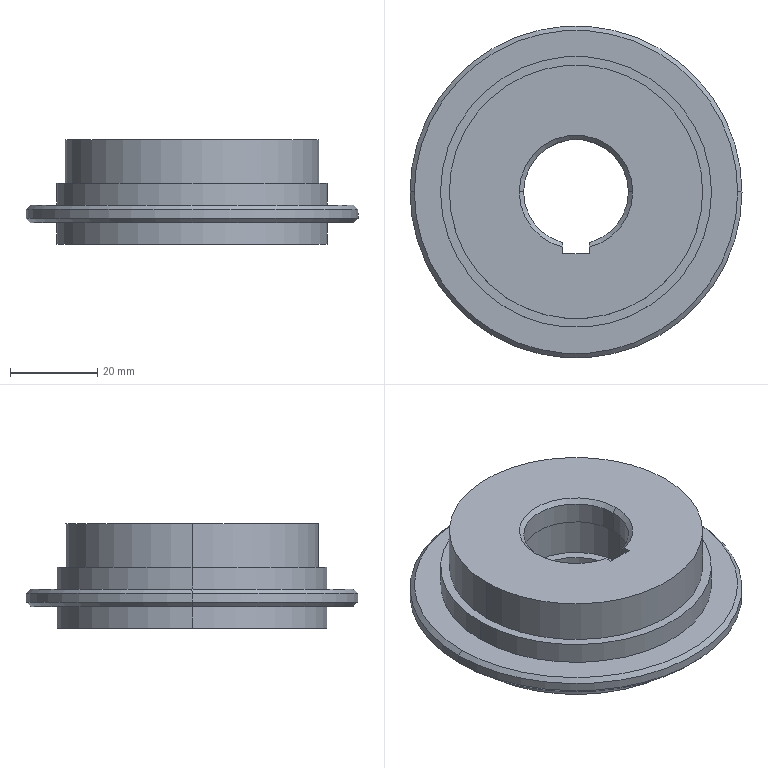Part | SolidWorks | features MirrorStock 1 | 2 solids | 49 faces | box 76 x 76 x 24 mm | volume 54312 mm3 | cylinder 25 | plane 14 | cone 10 | commonest cylinder face diameters 24 x6 58 x6 62 x4 28 x3 49 x2 52 x2
STEP:
#1=CARTESIAN_POINT('',(-12.,0.,21.));
#2=VERTEX_POINT('',#1);
#3=CARTESIAN_POINT('',(12.,0.,21.));
#4=VERTEX_POINT('',#3);
#5=CARTESIAN_POINT('',(0.,0.,21.));
#6=DIRECTION('',(0.,0.,-1.));
#7=DIRECTION('',(1.,0.,0.));
#8=AXIS2_PLACEMENT_3D('',#5,#6,#7);
#9=CIRCLE('',#8,12.);
#10=EDGE_CURVE('',#2,#4,#9,.T.);
#11=ORIENTED_EDGE('',*,*,#10,.T.);
#12=CARTESIAN_POINT('',(13.,0.,22.));
#13=VERTEX_POINT('',#12);
#14=CARTESIAN_POINT('',(13.,0.,22.));
#15=DIRECTION('',(0.7071,0.,0.7071));
#16=VECTOR('',#15,1000.);
#17=LINE('',#14,#16);
#18=EDGE_CURVE('',#4,#13,#17,.T.);
#19=ORIENTED_EDGE('',*,*,#18,.T.);
#20=CARTESIAN_POINT('',(-13.,0.,22.));
#21=VERTEX_POINT('',#20);
#22=CARTESIAN_POINT('',(0.,0.,22.));
#23=DIRECTION('',(0.,0.,1.));
#24=DIRECTION('',(1.,0.,0.));
#25=AXIS2_PLACEMENT_3D('',#22,#23,#24);
#26=CIRCLE('',#25,13.);
#27=EDGE_CURVE('',#13,#21,#26,.T.);
#28=ORIENTED_EDGE('',*,*,#27,.T.);
#29=CARTESIAN_POINT('',(-13.,0.,22.));
#30=DIRECTION('',(-0.7071,0.,0.7071));
#31=VECTOR('',#30,1000.);
#32=LINE('',#29,#31);
#33=EDGE_CURVE('',#2,#21,#32,.T.);
#34=ORIENTED_EDGE('',*,*,#33,.F.);
#35=EDGE_LOOP('',(#11,#19,#28,#34));
#36=FACE_OUTER_BOUND('',#35,.T.);
#37=CARTESIAN_POINT('',(0.,0.,22.));
#38=DIRECTION('',(0.,0.,1.));
#39=DIRECTION('',(-1.,0.,0.));
#40=AXIS2_PLACEMENT_3D('',#37,#38,#39);
#41=CONICAL_SURFACE('',#40,13.,0.7854);
#42=ADVANCED_FACE('',(#36),#41,.F.);
#43=CARTESIAN_POINT('',(-3.,-11.619,21.));
#44=VERTEX_POINT('',#43);
#45=CARTESIAN_POINT('',(0.,0.,21.));
#46=DIRECTION('',(0.,0.,-1.));
#47=DIRECTION('',(1.,0.,0.));
#48=AXIS2_PLACEMENT_3D('',#45,#46,#47);
#49=CIRCLE('',#48,12.);
#50=EDGE_CURVE('',#44,#2,#49,.T.);
#51=ORIENTED_EDGE('',*,*,#50,.T.);
#52=ORIENTED_EDGE('',*,*,#33,.T.);
#53=CARTESIAN_POINT('',(-3.,-12.649,22.));
#54=VERTEX_POINT('',#53);
#55=CARTESIAN_POINT('',(0.,0.,22.));
#56=DIRECTION('',(0.,0.,1.));
#57=DIRECTION('',(1.,0.,0.));
#58=AXIS2_PLACEMENT_3D('',#55,#56,#57);
#59=CIRCLE('',#58,13.);
#60=EDGE_CURVE('',#21,#54,#59,.T.);
#61=ORIENTED_EDGE('',*,*,#60,.T.);
#62=CARTESIAN_POINT('',(-3.,-12.649,22.));
#63=CARTESIAN_POINT('',(-3.,-12.306,21.666));
#64=CARTESIAN_POINT('',(-3.,-11.963,21.333));
#65=CARTESIAN_POINT('',(-3.,-11.619,21.));
#66=B_SPLINE_CURVE_WITH_KNOTS('',3,(#62,#63,#64,#65),.UNSPECIFIED.,.F.,.F.,(4,4),(0.,0.001436),.UNSPECIFIED.);
#67=EDGE_CURVE('',#54,#44,#66,.T.);
#68=ORIENTED_EDGE('',*,*,#67,.T.);
#69=EDGE_LOOP('',(#51,#52,#61,#68));
#70=FACE_OUTER_BOUND('',#69,.T.);
#71=CARTESIAN_POINT('',(0.,0.,22.));
#72=DIRECTION('',(0.,0.,1.));
#73=DIRECTION('',(-1.,0.,0.));
#74=AXIS2_PLACEMENT_3D('',#71,#72,#73);
#75=CONICAL_SURFACE('',#74,13.,0.7854);
#76=ADVANCED_FACE('',(#70),#75,.F.);
#77=CARTESIAN_POINT('',(12.,0.,1.));
#78=VERTEX_POINT('',#77);
#79=CARTESIAN_POINT('',(-12.,0.,1.));
#80=VERTEX_POINT('',#79);
#81=CARTESIAN_POINT('',(0.,0.,1.));
#82=DIRECTION('',(0.,0.,1.));
#83=DIRECTION('',(-1.,0.,0.));
#84=AXIS2_PLACEMENT_3D('',#81,#82,#83);
#85=CIRCLE('',#84,12.);
#86=EDGE_CURVE('',#78,#80,#85,.T.);
#87=ORIENTED_EDGE('',*,*,#86,.T.);
#88=CARTESIAN_POINT('',(-13.,0.,0.));
#89=VERTEX_POINT('',#88);
#90=CARTESIAN_POINT('',(-12.,0.,1.));
#91=DIRECTION('',(-0.7071,0.,-0.7071));
#92=VECTOR('',#91,1000.);
#93=LINE('',#90,#92);
#94=EDGE_CURVE('',#80,#89,#93,.T.);
#95=ORIENTED_EDGE('',*,*,#94,.T.);
#96=CARTESIAN_POINT('',(13.,0.,0.));
#97=VERTEX_POINT('',#96);
#98=CARTESIAN_POINT('',(0.,0.,0.));
#99=DIRECTION('',(0.,0.,-1.));
#100=DIRECTION('',(-1.,0.,0.));
#101=AXIS2_PLACEMENT_3D('',#98,#99,#100);
#102=CIRCLE('',#101,13.);
#103=EDGE_CURVE('',#89,#97,#102,.T.);
#104=ORIENTED_EDGE('',*,*,#103,.T.);
#105=CARTESIAN_POINT('',(12.,0.,1.));
#106=DIRECTION('',(0.7071,0.,-0.7071));
#107=VECTOR('',#106,1000.);
#108=LINE('',#105,#107);
#109=EDGE_CURVE('',#78,#97,#108,.T.);
#110=ORIENTED_EDGE('',*,*,#109,.F.);
#111=EDGE_LOOP('',(#87,#95,#104,#110));
#112=FACE_OUTER_BOUND('',#111,.T.);
#113=CARTESIAN_POINT('',(0.,0.,1.));
#114=DIRECTION('',(0.,0.,-1.));
#115=DIRECTION('',(1.,0.,0.));
#116=AXIS2_PLACEMENT_3D('',#113,#114,#115);
#117=CONICAL_SURFACE('',#116,12.,0.7854);
#118=ADVANCED_FACE('',(#112),#117,.F.);
#119=CARTESIAN_POINT('',(3.,-11.619,1.));
#120=VERTEX_POINT('',#119);
#121=CARTESIAN_POINT('',(0.,0.,1.));
#122=DIRECTION('',(0.,0.,1.));
#123=DIRECTION('',(-1.,0.,0.));
#124=AXIS2_PLACEMENT_3D('',#121,#122,#123);
#125=CIRCLE('',#124,12.);
#126=EDGE_CURVE('',#120,#78,#125,.T.);
#127=ORIENTED_EDGE('',*,*,#126,.T.);
#128=ORIENTED_EDGE('',*,*,#109,.T.);
#129=CARTESIAN_POINT('',(3.,-12.649,0.));
#130=VERTEX_POINT('',#129);
#131=CARTESIAN_POINT('',(0.,0.,0.));
#132=DIRECTION('',(0.,0.,-1.));
#133=DIRECTION('',(-1.,0.,0.));
#134=AXIS2_PLACEMENT_3D('',#131,#132,#133);
#135=CIRCLE('',#134,13.);
#136=EDGE_CURVE('',#97,#130,#135,.T.);
#137=ORIENTED_EDGE('',*,*,#136,.T.);
#138=CARTESIAN_POINT('',(3.,-12.649,0.));
#139=CARTESIAN_POINT('',(3.,-12.306,0.3337));
#140=CARTESIAN_POINT('',(3.,-11.963,0.6671));
#141=CARTESIAN_POINT('',(3.,-11.619,1.));
#142=B_SPLINE_CURVE_WITH_KNOTS('',3,(#138,#139,#140,#141),.UNSPECIFIED.,.F.,.F.,(4,4),(0.,0.001436),.UNSPECIFIED.);
#143=EDGE_CURVE('',#130,#120,#142,.T.);
#144=ORIENTED_EDGE('',*,*,#143,.T.);
#145=EDGE_LOOP('',(#127,#128,#137,#144));
#146=FACE_OUTER_BOUND('',#145,.T.);
#147=CARTESIAN_POINT('',(0.,0.,1.));
#148=DIRECTION('',(0.,0.,-1.));
#149=DIRECTION('',(1.,0.,0.));
#150=AXIS2_PLACEMENT_3D('',#147,#148,#149);
#151=CONICAL_SURFACE('',#150,12.,0.7854);
#152=ADVANCED_FACE('',(#146),#151,.F.);
#153=CARTESIAN_POINT('',(-29.,0.,22.));
#154=VERTEX_POINT('',#153);
#155=CARTESIAN_POINT('',(29.,0.,22.));
#156=VERTEX_POINT('',#155);
#157=CARTESIAN_POINT('',(0.,0.,22.));
#158=DIRECTION('',(0.,0.,1.));
#159=DIRECTION('',(1.,0.,0.));
#160=AXIS2_PLACEMENT_3D('',#157,#158,#159);
#161=CIRCLE('',#160,29.);
#162=EDGE_CURVE('',#154,#156,#161,.T.);
#163=ORIENTED_EDGE('',*,*,#162,.F.);
#164=CARTESIAN_POINT('',(-29.,0.,7.5));
#165=VERTEX_POINT('',#164);
#166=CARTESIAN_POINT('',(-29.,0.,0.));
#167=DIRECTION('',(0.,0.,-1.));
#168=VECTOR('',#167,1000.);
#169=LINE('',#166,#168);
#170=EDGE_CURVE('',#154,#165,#169,.T.);
#171=ORIENTED_EDGE('',*,*,#170,.T.);
#172=CARTESIAN_POINT('',(29.,0.,7.5));
#173=VERTEX_POINT('',#172);
#174=CARTESIAN_POINT('',(0.,0.,7.5));
#175=DIRECTION('',(0.,0.,1.));
#176=DIRECTION('',(1.,0.,0.));
#177=AXIS2_PLACEMENT_3D('',#174,#175,#176);
#178=CIRCLE('',#177,29.);
#179=EDGE_CURVE('',#165,#173,#178,.T.);
#180=ORIENTED_EDGE('',*,*,#179,.T.);
#181=CARTESIAN_POINT('',(29.,0.,0.));
#182=DIRECTION('',(0.,0.,-1.));
#183=VECTOR('',#182,1000.);
#184=LINE('',#181,#183);
#185=EDGE_CURVE('',#156,#173,#184,.T.);
#186=ORIENTED_EDGE('',*,*,#185,.F.);
#187=EDGE_LOOP('',(#163,#171,#180,#186));
#188=FACE_OUTER_BOUND('',#187,.T.);
#189=CARTESIAN_POINT('',(0.,0.,0.));
#190=DIRECTION('',(0.,0.,-1.));
#191=DIRECTION('',(1.,0.,0.));
#192=AXIS2_PLACEMENT_3D('',#189,#190,#191);
#193=CYLINDRICAL_SURFACE('',#192,29.);
#194=ADVANCED_FACE('',(#188),#193,.T.);
#195=CARTESIAN_POINT('',(-24.5,0.,7.5));
#196=VERTEX_POINT('',#195);
#197=CARTESIAN_POINT('',(24.5,0.,7.5));
#198=VERTEX_POINT('',#197);
#199=CARTESIAN_POINT('',(0.,0.,7.5));
#200=DIRECTION('',(0.,0.,1.));
#201=DIRECTION('',(1.,0.,0.));
#202=AXIS2_PLACEMENT_3D('',#199,#200,#201);
#203=CIRCLE('',#202,24.5);
#204=EDGE_CURVE('',#196,#198,#203,.T.);
#205=ORIENTED_EDGE('',*,*,#204,.F.);
#206=CARTESIAN_POINT('',(-24.5,0.,0.));
#207=VERTEX_POINT('',#206);
#208=CARTESIAN_POINT('',(-24.5,0.,0.));
#209=DIRECTION('',(0.,0.,-1.));
#210=VECTOR('',#209,1000.);
#211=LINE('',#208,#210);
#212=EDGE_CURVE('',#196,#207,#211,.T.);
#213=ORIENTED_EDGE('',*,*,#212,.T.);
#214=CARTESIAN_POINT('',(24.5,0.,0.));
#215=VERTEX_POINT('',#214);
#216=CARTESIAN_POINT('',(0.,0.,0.));
#217=DIRECTION('',(0.,0.,1.));
#218=DIRECTION('',(1.,0.,0.));
#219=AXIS2_PLACEMENT_3D('',#216,#217,#218);
#220=CIRCLE('',#219,24.5);
#221=EDGE_CURVE('',#207,#215,#220,.T.);
#222=ORIENTED_EDGE('',*,*,#221,.T.);
#223=CARTESIAN_POINT('',(24.5,0.,0.));
#224=DIRECTION('',(0.,0.,-1.));
#225=VECTOR('',#224,1000.);
#226=LINE('',#223,#225);
#227=EDGE_CURVE('',#198,#215,#226,.T.);
#228=ORIENTED_EDGE('',*,*,#227,.F.);
#229=EDGE_LOOP('',(#205,#213,#222,#228));
#230=FACE_OUTER_BOUND('',#229,.T.);
#231=CARTESIAN_POINT('',(0.,0.,0.));
#232=DIRECTION('',(0.,0.,-1.));
#233=DIRECTION('',(1.,0.,0.));
#234=AXIS2_PLACEMENT_3D('',#231,#232,#233);
#235=CYLINDRICAL_SURFACE('',#234,24.5);
#236=ADVANCED_FACE('',(#230),#235,.T.);
#237=CARTESIAN_POINT('',(12.,0.,6.));
#238=VERTEX_POINT('',#237);
#239=CARTESIAN_POINT('',(-12.,0.,6.));
#240=VERTEX_POINT('',#239);
#241=CARTESIAN_POINT('',(0.,0.,6.));
#242=DIRECTION('',(0.,0.,1.));
#243=DIRECTION('',(1.,0.,0.));
#244=AXIS2_PLACEMENT_3D('',#241,#242,#243);
#245=CIRCLE('',#244,12.);
#246=EDGE_CURVE('',#238,#240,#245,.T.);
#247=ORIENTED_EDGE('',*,*,#246,.T.);
#248=CARTESIAN_POINT('',(-12.,0.,0.));
#249=DIRECTION('',(0.,0.,-1.));
#250=VECTOR('',#249,1000.);
#251=LINE('',#248,#250);
#252=EDGE_CURVE('',#240,#80,#251,.T.);
#253=ORIENTED_EDGE('',*,*,#252,.T.);
#254=ORIENTED_EDGE('',*,*,#86,.F.);
#255=CARTESIAN_POINT('',(12.,0.,0.));
#256=DIRECTION('',(0.,0.,-1.));
#257=VECTOR('',#256,1000.);
#258=LINE('',#255,#257);
#259=EDGE_CURVE('',#238,#78,#258,.T.);
#260=ORIENTED_EDGE('',*,*,#259,.F.);
#261=EDGE_LOOP('',(#247,#253,#254,#260));
#262=FACE_OUTER_BOUND('',#261,.T.);
#263=CARTESIAN_POINT('',(0.,0.,0.));
#264=DIRECTION('',(0.,0.,-1.));
#265=DIRECTION('',(1.,0.,0.));
#266=AXIS2_PLACEMENT_3D('',#263,#264,#265);
#267=CYLINDRICAL_SURFACE('',#266,12.);
#268=ADVANCED_FACE('',(#262),#267,.F.);
#269=CARTESIAN_POINT('',(3.,-11.619,6.));
#270=VERTEX_POINT('',#269);
#271=CARTESIAN_POINT('',(0.,0.,6.));
#272=DIRECTION('',(0.,0.,1.));
#273=DIRECTION('',(1.,0.,0.));
#274=AXIS2_PLACEMENT_3D('',#271,#272,#273);
#275=CIRCLE('',#274,12.);
#276=EDGE_CURVE('',#270,#238,#275,.T.);
#277=ORIENTED_EDGE('',*,*,#276,.T.);
#278=ORIENTED_EDGE('',*,*,#259,.T.);
#279=ORIENTED_EDGE('',*,*,#126,.F.);
#280=CARTESIAN_POINT('',(3.,-11.619,0.));
#281=DIRECTION('',(0.,0.,-1.));
#282=VECTOR('',#281,1000.);
#283=LINE('',#280,#282);
#284=EDGE_CURVE('',#270,#120,#283,.T.);
#285=ORIENTED_EDGE('',*,*,#284,.F.);
#286=EDGE_LOOP('',(#277,#278,#279,#285));
#287=FACE_OUTER_BOUND('',#286,.T.);
#288=CARTESIAN_POINT('',(0.,0.,0.));
#289=DIRECTION('',(0.,0.,-1.));
#290=DIRECTION('',(1.,0.,0.));
#291=AXIS2_PLACEMENT_3D('',#288,#289,#290);
#292=CYLINDRICAL_SURFACE('',#291,12.);
#293=ADVANCED_FACE('',(#287),#292,.F.);
#294=CARTESIAN_POINT('',(14.,0.,16.));
#295=VERTEX_POINT('',#294);
#296=CARTESIAN_POINT('',(-14.,0.,16.));
#297=VERTEX_POINT('',#296);
#298=CARTESIAN_POINT('',(0.,0.,16.));
#299=DIRECTION('',(0.,0.,1.));
#300=DIRECTION('',(1.,0.,0.));
#301=AXIS2_PLACEMENT_3D('',#298,#299,#300);
#302=CIRCLE('',#301,14.);
#303=EDGE_CURVE('',#295,#297,#302,.T.);
#304=ORIENTED_EDGE('',*,*,#303,.T.);
#305=CARTESIAN_POINT('',(-14.,0.,6.));
#306=VERTEX_POINT('',#305);
#307=CARTESIAN_POINT('',(-14.,0.,0.));
#308=DIRECTION('',(0.,0.,-1.));
#309=VECTOR('',#308,1000.);
#310=LINE('',#307,#309);
#311=EDGE_CURVE('',#297,#306,#310,.T.);
#312=ORIENTED_EDGE('',*,*,#311,.T.);
#313=CARTESIAN_POINT('',(14.,0.,6.));
#314=VERTEX_POINT('',#313);
#315=CARTESIAN_POINT('',(0.,0.,6.));
#316=DIRECTION('',(0.,0.,1.));
#317=DIRECTION('',(1.,0.,0.));
#318=AXIS2_PLACEMENT_3D('',#315,#316,#317);
#319=CIRCLE('',#318,14.);
#320=EDGE_CURVE('',#314,#306,#319,.T.);
#321=ORIENTED_EDGE('',*,*,#320,.F.);
#322=CARTESIAN_POINT('',(14.,0.,0.));
#323=DIRECTION('',(0.,0.,-1.));
#324=VECTOR('',#323,1000.);
#325=LINE('',#322,#324);
#326=EDGE_CURVE('',#295,#314,#325,.T.);
#327=ORIENTED_EDGE('',*,*,#326,.F.);
#328=EDGE_LOOP('',(#304,#312,#321,#327));
#329=FACE_OUTER_BOUND('',#328,.T.);
#330=CARTESIAN_POINT('',(0.,0.,0.));
#331=DIRECTION('',(0.,0.,-1.));
#332=DIRECTION('',(1.,0.,0.));
#333=AXIS2_PLACEMENT_3D('',#330,#331,#332);
#334=CYLINDRICAL_SURFACE('',#333,14.);
#335=ADVANCED_FACE('',(#329),#334,.F.);
#336=CARTESIAN_POINT('',(3.,-13.675,16.));
#337=VERTEX_POINT('',#336);
#338=CARTESIAN_POINT('',(0.,0.,16.));
#339=DIRECTION('',(0.,0.,1.));
#340=DIRECTION('',(1.,0.,0.));
#341=AXIS2_PLACEMENT_3D('',#338,#339,#340);
#342=CIRCLE('',#341,14.);
#343=EDGE_CURVE('',#337,#295,#342,.T.);
#344=ORIENTED_EDGE('',*,*,#343,.T.);
#345=ORIENTED_EDGE('',*,*,#326,.T.);
#346=CARTESIAN_POINT('',(3.,-13.675,6.));
#347=VERTEX_POINT('',#346);
#348=CARTESIAN_POINT('',(0.,0.,6.));
#349=DIRECTION('',(0.,0.,1.));
#350=DIRECTION('',(1.,0.,0.));
#351=AXIS2_PLACEMENT_3D('',#348,#349,#350);
#352=CIRCLE('',#351,14.);
#353=EDGE_CURVE('',#347,#314,#352,.T.);
#354=ORIENTED_EDGE('',*,*,#353,.F.);
#355=CARTESIAN_POINT('',(3.,-13.675,0.));
#356=DIRECTION('',(0.,0.,-1.));
#357=VECTOR('',#356,1000.);
#358=LINE('',#355,#357);
#359=EDGE_CURVE('',#337,#347,#358,.T.);
#360=ORIENTED_EDGE('',*,*,#359,.F.);
#361=EDGE_LOOP('',(#344,#345,#354,#360));
#362=FACE_OUTER_BOUND('',#361,.T.);
#363=CARTESIAN_POINT('',(0.,0.,0.));
#364=DIRECTION('',(0.,0.,-1.));
#365=DIRECTION('',(1.,0.,0.));
#366=AXIS2_PLACEMENT_3D('',#363,#364,#365);
#367=CYLINDRICAL_SURFACE('',#366,14.);
#368=ADVANCED_FACE('',(#362),#367,.F.);
#369=ORIENTED_EDGE('',*,*,#10,.F.);
#370=CARTESIAN_POINT('',(-12.,0.,16.));
#371=VERTEX_POINT('',#370);
#372=CARTESIAN_POINT('',(-12.,0.,0.));
#373=DIRECTION('',(0.,0.,-1.));
#374=VECTOR('',#373,1000.);
#375=LINE('',#372,#374);
#376=EDGE_CURVE('',#2,#371,#375,.T.);
#377=ORIENTED_EDGE('',*,*,#376,.T.);
#378=CARTESIAN_POINT('',(12.,0.,16.));
#379=VERTEX_POINT('',#378);
#380=CARTESIAN_POINT('',(0.,0.,16.));
#381=DIRECTION('',(0.,0.,1.));
#382=DIRECTION('',(1.,0.,0.));
#383=AXIS2_PLACEMENT_3D('',#380,#381,#382);
#384=CIRCLE('',#383,12.);
#385=EDGE_CURVE('',#379,#371,#384,.T.);
#386=ORIENTED_EDGE('',*,*,#385,.F.);
#387=CARTESIAN_POINT('',(12.,0.,0.));
#388=DIRECTION('',(0.,0.,-1.));
#389=VECTOR('',#388,1000.);
#390=LINE('',#387,#389);
#391=EDGE_CURVE('',#4,#379,#390,.T.);
#392=ORIENTED_EDGE('',*,*,#391,.F.);
#393=EDGE_LOOP('',(#369,#377,#386,#392));
#394=FACE_OUTER_BOUND('',#393,.T.);
#395=CARTESIAN_POINT('',(0.,0.,0.));
#396=DIRECTION('',(0.,0.,-1.));
#397=DIRECTION('',(1.,0.,0.));
#398=AXIS2_PLACEMENT_3D('',#395,#396,#397);
#399=CYLINDRICAL_SURFACE('',#398,12.);
#400=ADVANCED_FACE('',(#394),#399,.F.);
#401=CARTESIAN_POINT('',(3.,-11.619,21.));
#402=VERTEX_POINT('',#401);
#403=CARTESIAN_POINT('',(0.,0.,21.));
#404=DIRECTION('',(0.,0.,-1.));
#405=DIRECTION('',(1.,0.,0.));
#406=AXIS2_PLACEMENT_3D('',#403,#404,#405);
#407=CIRCLE('',#406,12.);
#408=EDGE_CURVE('',#4,#402,#407,.T.);
#409=ORIENTED_EDGE('',*,*,#408,.F.);
#410=ORIENTED_EDGE('',*,*,#391,.T.);
#411=CARTESIAN_POINT('',(3.,-11.619,16.));
#412=VERTEX_POINT('',#411);
#413=CARTESIAN_POINT('',(0.,0.,16.));
#414=DIRECTION('',(0.,0.,1.));
#415=DIRECTION('',(1.,0.,0.));
#416=AXIS2_PLACEMENT_3D('',#413,#414,#415);
#417=CIRCLE('',#416,12.);
#418=EDGE_CURVE('',#412,#379,#417,.T.);
#419=ORIENTED_EDGE('',*,*,#418,.F.);
#420=CARTESIAN_POINT('',(3.,-11.619,0.));
#421=DIRECTION('',(0.,0.,-1.));
#422=VECTOR('',#421,1000.);
#423=LINE('',#420,#422);
#424=EDGE_CURVE('',#402,#412,#423,.T.);
#425=ORIENTED_EDGE('',*,*,#424,.F.);
#426=EDGE_LOOP('',(#409,#410,#419,#425));
#427=FACE_OUTER_BOUND('',#426,.T.);
#428=CARTESIAN_POINT('',(0.,0.,0.));
#429=DIRECTION('',(0.,0.,-1.));
#430=DIRECTION('',(1.,0.,0.));
#431=AXIS2_PLACEMENT_3D('',#428,#429,#430);
#432=CYLINDRICAL_SURFACE('',#431,12.);
#433=ADVANCED_FACE('',(#427),#432,.F.);
#434=CARTESIAN_POINT('',(0.,0.,22.));
#435=DIRECTION('',(0.,0.,1.));
#436=DIRECTION('',(1.,0.,0.));
#437=AXIS2_PLACEMENT_3D('',#434,#435,#436);
#438=CIRCLE('',#437,29.);
#439=EDGE_CURVE('',#156,#154,#438,.T.);
#440=ORIENTED_EDGE('',*,*,#439,.T.);
#441=ORIENTED_EDGE('',*,*,#162,.T.);
#442=EDGE_LOOP('',(#440,#441));
#443=FACE_OUTER_BOUND('',#442,.T.);
#444=CARTESIAN_POINT('',(3.,-12.649,22.));
#445=VERTEX_POINT('',#444);
#446=CARTESIAN_POINT('',(3.,-14.2,22.));
#447=VERTEX_POINT('',#446);
#448=CARTESIAN_POINT('',(3.,-14.2,22.));
#449=DIRECTION('',(0.,-1.,0.));
#450=VECTOR('',#449,1000.);
#451=LINE('',#448,#450);
#452=EDGE_CURVE('',#445,#447,#451,.T.);
#453=ORIENTED_EDGE('',*,*,#452,.T.);
#454=CARTESIAN_POINT('',(-3.,-14.2,22.));
#455=VERTEX_POINT('',#454);
#456=CARTESIAN_POINT('',(-3.,-14.2,22.));
#457=DIRECTION('',(-1.,0.,0.));
#458=VECTOR('',#457,1000.);
#459=LINE('',#456,#458);
#460=EDGE_CURVE('',#447,#455,#459,.T.);
#461=ORIENTED_EDGE('',*,*,#460,.T.);
#462=CARTESIAN_POINT('',(-3.,-14.2,22.));
#463=DIRECTION('',(0.,1.,0.));
#464=VECTOR('',#463,1000.);
#465=LINE('',#462,#464);
#466=EDGE_CURVE('',#455,#54,#465,.T.);
#467=ORIENTED_EDGE('',*,*,#466,.T.);
#468=ORIENTED_EDGE('',*,*,#60,.F.);
#469=ORIENTED_EDGE('',*,*,#27,.F.);
#470=CARTESIAN_POINT('',(0.,0.,22.));
#471=DIRECTION('',(0.,0.,1.));
#472=DIRECTION('',(1.,0.,0.));
#473=AXIS2_PLACEMENT_3D('',#470,#471,#472);
#474=CIRCLE('',#473,13.);
#475=EDGE_CURVE('',#445,#13,#474,.T.);
#476=ORIENTED_EDGE('',*,*,#475,.F.);
#477=EDGE_LOOP('',(#453,#461,#467,#468,#469,#476));
#478=FACE_BOUND('',#477,.T.);
#479=CARTESIAN_POINT('',(-29.,0.,22.));
#480=DIRECTION('',(0.,0.,-1.));
#481=DIRECTION('',(1.,0.,0.));
#482=AXIS2_PLACEMENT_3D('',#479,#480,#481);
#483=PLANE('',#482);
#484=ADVANCED_FACE('',(#443,#478),#483,.F.);
#485=ORIENTED_EDGE('',*,*,#376,.F.);
#486=ORIENTED_EDGE('',*,*,#50,.F.);
#487=CARTESIAN_POINT('',(-3.,-11.619,16.));
#488=VERTEX_POINT('',#487);
#489=CARTESIAN_POINT('',(-3.,-11.619,0.));
#490=DIRECTION('',(0.,0.,1.));
#491=VECTOR('',#490,1000.);
#492=LINE('',#489,#491);
#493=EDGE_CURVE('',#488,#44,#492,.T.);
#494=ORIENTED_EDGE('',*,*,#493,.F.);
#495=CARTESIAN_POINT('',(0.,0.,16.));
#496=DIRECTION('',(0.,0.,1.));
#497=DIRECTION('',(1.,0.,0.));
#498=AXIS2_PLACEMENT_3D('',#495,#496,#497);
#499=CIRCLE('',#498,12.);
#500=EDGE_CURVE('',#371,#488,#499,.T.);
#501=ORIENTED_EDGE('',*,*,#500,.F.);
#502=EDGE_LOOP('',(#485,#486,#494,#501));
#503=FACE_OUTER_BOUND('',#502,.T.);
#504=CARTESIAN_POINT('',(0.,0.,0.));
#505=DIRECTION('',(0.,0.,-1.));
#506=DIRECTION('',(1.,0.,0.));
#507=AXIS2_PLACEMENT_3D('',#504,#505,#506);
#508=CYLINDRICAL_SURFACE('',#507,12.);
#509=ADVANCED_FACE('',(#503),#508,.F.);
#510=ORIENTED_EDGE('',*,*,#418,.T.);
#511=ORIENTED_EDGE('',*,*,#385,.T.);
#512=ORIENTED_EDGE('',*,*,#500,.T.);
#513=CARTESIAN_POINT('',(-3.,-13.675,16.));
#514=VERTEX_POINT('',#513);
#515=CARTESIAN_POINT('',(-3.,0.,16.));
#516=DIRECTION('',(0.,1.,0.));
#517=VECTOR('',#516,1000.);
#518=LINE('',#515,#517);
#519=EDGE_CURVE('',#514,#488,#518,.T.);
#520=ORIENTED_EDGE('',*,*,#519,.F.);
#521=CARTESIAN_POINT('',(0.,0.,16.));
#522=DIRECTION('',(0.,0.,1.));
#523=DIRECTION('',(1.,0.,0.));
#524=AXIS2_PLACEMENT_3D('',#521,#522,#523);
#525=CIRCLE('',#524,14.);
#526=EDGE_CURVE('',#297,#514,#525,.T.);
#527=ORIENTED_EDGE('',*,*,#526,.F.);
#528=ORIENTED_EDGE('',*,*,#303,.F.);
#529=ORIENTED_EDGE('',*,*,#343,.F.);
#530=CARTESIAN_POINT('',(3.,0.,16.));
#531=DIRECTION('',(0.,-1.,0.));
#532=VECTOR('',#531,1000.);
#533=LINE('',#530,#532);
#534=EDGE_CURVE('',#412,#337,#533,.T.);
#535=ORIENTED_EDGE('',*,*,#534,.F.);
#536=EDGE_LOOP('',(#510,#511,#512,#520,#527,#528,#529,#535));
#537=FACE_OUTER_BOUND('',#536,.T.);
#538=CARTESIAN_POINT('',(-12.,0.,16.));
#539=DIRECTION('',(0.,0.,1.));
#540=DIRECTION('',(-1.,0.,0.));
#541=AXIS2_PLACEMENT_3D('',#538,#539,#540);
#542=PLANE('',#541);
#543=ADVANCED_FACE('',(#537),#542,.F.);
#544=ORIENTED_EDGE('',*,*,#311,.F.);
#545=ORIENTED_EDGE('',*,*,#526,.T.);
#546=CARTESIAN_POINT('',(-3.,-13.675,6.));
#547=VERTEX_POINT('',#546);
#548=CARTESIAN_POINT('',(-3.,-13.675,0.));
#549=DIRECTION('',(0.,0.,1.));
#550=VECTOR('',#549,1000.);
#551=LINE('',#548,#550);
#552=EDGE_CURVE('',#547,#514,#551,.T.);
#553=ORIENTED_EDGE('',*,*,#552,.F.);
#554=CARTESIAN_POINT('',(0.,0.,6.));
#555=DIRECTION('',(0.,0.,1.));
#556=DIRECTION('',(1.,0.,0.));
#557=AXIS2_PLACEMENT_3D('',#554,#555,#556);
#558=CIRCLE('',#557,14.);
#559=EDGE_CURVE('',#306,#547,#558,.T.);
#560=ORIENTED_EDGE('',*,*,#559,.F.);
#561=EDGE_LOOP('',(#544,#545,#553,#560));
#562=FACE_OUTER_BOUND('',#561,.T.);
#563=CARTESIAN_POINT('',(0.,0.,0.));
#564=DIRECTION('',(0.,0.,-1.));
#565=DIRECTION('',(1.,0.,0.));
#566=AXIS2_PLACEMENT_3D('',#563,#564,#565);
#567=CYLINDRICAL_SURFACE('',#566,14.);
#568=ADVANCED_FACE('',(#562),#567,.F.);
#569=ORIENTED_EDGE('',*,*,#353,.T.);
#570=ORIENTED_EDGE('',*,*,#320,.T.);
#571=ORIENTED_EDGE('',*,*,#559,.T.);
#572=CARTESIAN_POINT('',(-3.,-11.619,6.));
#573=VERTEX_POINT('',#572);
#574=CARTESIAN_POINT('',(-3.,0.,6.));
#575=DIRECTION('',(0.,-1.,0.));
#576=VECTOR('',#575,1000.);
#577=LINE('',#574,#576);
#578=EDGE_CURVE('',#573,#547,#577,.T.);
#579=ORIENTED_EDGE('',*,*,#578,.F.);
#580=CARTESIAN_POINT('',(0.,0.,6.));
#581=DIRECTION('',(0.,0.,1.));
#582=DIRECTION('',(1.,0.,0.));
#583=AXIS2_PLACEMENT_3D('',#580,#581,#582);
#584=CIRCLE('',#583,12.);
#585=EDGE_CURVE('',#240,#573,#584,.T.);
#586=ORIENTED_EDGE('',*,*,#585,.F.);
#587=ORIENTED_EDGE('',*,*,#246,.F.);
#588=ORIENTED_EDGE('',*,*,#276,.F.);
#589=CARTESIAN_POINT('',(3.,0.,6.));
#590=DIRECTION('',(0.,1.,0.));
#591=VECTOR('',#590,1000.);
#592=LINE('',#589,#591);
#593=EDGE_CURVE('',#347,#270,#592,.T.);
#594=ORIENTED_EDGE('',*,*,#593,.F.);
#595=EDGE_LOOP('',(#569,#570,#571,#579,#586,#587,#588,#594));
#596=FACE_OUTER_BOUND('',#595,.T.);
#597=CARTESIAN_POINT('',(-14.,0.,6.));
#598=DIRECTION('',(0.,0.,-1.));
#599=DIRECTION('',(1.,0.,0.));
#600=AXIS2_PLACEMENT_3D('',#597,#598,#599);
#601=PLANE('',#600);
#602=ADVANCED_FACE('',(#596),#601,.F.);
#603=ORIENTED_EDGE('',*,*,#252,.F.);
#604=ORIENTED_EDGE('',*,*,#585,.T.);
#605=CARTESIAN_POINT('',(-3.,-11.619,1.));
#606=VERTEX_POINT('',#605);
#607=CARTESIAN_POINT('',(-3.,-11.619,0.));
#608=DIRECTION('',(0.,0.,1.));
#609=VECTOR('',#608,1000.);
#610=LINE('',#607,#609);
#611=EDGE_CURVE('',#606,#573,#610,.T.);
#612=ORIENTED_EDGE('',*,*,#611,.F.);
#613=CARTESIAN_POINT('',(0.,0.,1.));
#614=DIRECTION('',(0.,0.,1.));
#615=DIRECTION('',(-1.,0.,0.));
#616=AXIS2_PLACEMENT_3D('',#613,#614,#615);
#617=CIRCLE('',#616,12.);
#618=EDGE_CURVE('',#80,#606,#617,.T.);
#619=ORIENTED_EDGE('',*,*,#618,.F.);
#620=EDGE_LOOP('',(#603,#604,#612,#619));
#621=FACE_OUTER_BOUND('',#620,.T.);
#622=CARTESIAN_POINT('',(0.,0.,0.));
#623=DIRECTION('',(0.,0.,-1.));
#624=DIRECTION('',(1.,0.,0.));
#625=AXIS2_PLACEMENT_3D('',#622,#623,#624);
#626=CYLINDRICAL_SURFACE('',#625,12.);
#627=ADVANCED_FACE('',(#621),#626,.F.);
#628=CARTESIAN_POINT('',(-3.,-14.2,0.));
#629=VERTEX_POINT('',#628);
#630=CARTESIAN_POINT('',(-3.,-12.649,0.));
#631=VERTEX_POINT('',#630);
#632=CARTESIAN_POINT('',(-3.,0.,0.));
#633=DIRECTION('',(0.,1.,0.));
#634=VECTOR('',#633,1000.);
#635=LINE('',#632,#634);
#636=EDGE_CURVE('',#629,#631,#635,.T.);
#637=ORIENTED_EDGE('',*,*,#636,.F.);
#638=CARTESIAN_POINT('',(3.,-14.2,0.));
#639=VERTEX_POINT('',#638);
#640=CARTESIAN_POINT('',(-12.,-14.2,0.));
#641=DIRECTION('',(-1.,0.,0.));
#642=VECTOR('',#641,1000.);
#643=LINE('',#640,#642);
#644=EDGE_CURVE('',#639,#629,#643,.T.);
#645=ORIENTED_EDGE('',*,*,#644,.F.);
#646=CARTESIAN_POINT('',(3.,0.,0.));
#647=DIRECTION('',(0.,-1.,0.));
#648=VECTOR('',#647,1000.);
#649=LINE('',#646,#648);
#650=EDGE_CURVE('',#130,#639,#649,.T.);
#651=ORIENTED_EDGE('',*,*,#650,.F.);
#652=ORIENTED_EDGE('',*,*,#136,.F.);
#653=ORIENTED_EDGE('',*,*,#103,.F.);
#654=CARTESIAN_POINT('',(0.,0.,0.));
#655=DIRECTION('',(0.,0.,-1.));
#656=DIRECTION('',(-1.,0.,0.));
#657=AXIS2_PLACEMENT_3D('',#654,#655,#656);
#658=CIRCLE('',#657,13.);
#659=EDGE_CURVE('',#631,#89,#658,.T.);
#660=ORIENTED_EDGE('',*,*,#659,.F.);
#661=EDGE_LOOP('',(#637,#645,#651,#652,#653,#660));
#662=FACE_BOUND('',#661,.T.);
#663=CARTESIAN_POINT('',(0.,0.,0.));
#664=DIRECTION('',(0.,0.,1.));
#665=DIRECTION('',(1.,0.,0.));
#666=AXIS2_PLACEMENT_3D('',#663,#664,#665);
#667=CIRCLE('',#666,24.5);
#668=EDGE_CURVE('',#215,#207,#667,.T.);
#669=ORIENTED_EDGE('',*,*,#668,.F.);
#670=ORIENTED_EDGE('',*,*,#221,.F.);
#671=EDGE_LOOP('',(#669,#670));
#672=FACE_OUTER_BOUND('',#671,.T.);
#673=CARTESIAN_POINT('',(-12.,0.,0.));
#674=DIRECTION('',(0.,0.,1.));
#675=DIRECTION('',(-1.,0.,0.));
#676=AXIS2_PLACEMENT_3D('',#673,#674,#675);
#677=PLANE('',#676);
#678=ADVANCED_FACE('',(#662,#672),#677,.F.);
#679=ORIENTED_EDGE('',*,*,#212,.F.);
#680=CARTESIAN_POINT('',(0.,0.,7.5));
#681=DIRECTION('',(0.,0.,1.));
#682=DIRECTION('',(1.,0.,0.));
#683=AXIS2_PLACEMENT_3D('',#680,#681,#682);
#684=CIRCLE('',#683,24.5);
#685=EDGE_CURVE('',#198,#196,#684,.T.);
#686=ORIENTED_EDGE('',*,*,#685,.F.);
#687=ORIENTED_EDGE('',*,*,#227,.T.);
#688=ORIENTED_EDGE('',*,*,#668,.T.);
#689=EDGE_LOOP('',(#679,#686,#687,#688));
#690=FACE_OUTER_BOUND('',#689,.T.);
#691=CARTESIAN_POINT('',(0.,0.,0.));
#692=DIRECTION('',(0.,0.,-1.));
#693=DIRECTION('',(1.,0.,0.));
#694=AXIS2_PLACEMENT_3D('',#691,#692,#693);
#695=CYLINDRICAL_SURFACE('',#694,24.5);
#696=ADVANCED_FACE('',(#690),#695,.T.);
#697=ORIENTED_EDGE('',*,*,#685,.T.);
#698=ORIENTED_EDGE('',*,*,#204,.T.);
#699=EDGE_LOOP('',(#697,#698));
#700=FACE_BOUND('',#699,.T.);
#701=CARTESIAN_POINT('',(0.,0.,7.5));
#702=DIRECTION('',(0.,0.,1.));
#703=DIRECTION('',(1.,0.,0.));
#704=AXIS2_PLACEMENT_3D('',#701,#702,#703);
#705=CIRCLE('',#704,29.);
#706=EDGE_CURVE('',#173,#165,#705,.T.);
#707=ORIENTED_EDGE('',*,*,#706,.F.);
#708=ORIENTED_EDGE('',*,*,#179,.F.);
#709=EDGE_LOOP('',(#707,#708));
#710=FACE_OUTER_BOUND('',#709,.T.);
#711=CARTESIAN_POINT('',(-24.5,0.,7.5));
#712=DIRECTION('',(0.,0.,1.));
#713=DIRECTION('',(-1.,0.,0.));
#714=AXIS2_PLACEMENT_3D('',#711,#712,#713);
#715=PLANE('',#714);
#716=ADVANCED_FACE('',(#700,#710),#715,.F.);
#717=ORIENTED_EDGE('',*,*,#170,.F.);
#718=ORIENTED_EDGE('',*,*,#439,.F.);
#719=ORIENTED_EDGE('',*,*,#185,.T.);
#720=ORIENTED_EDGE('',*,*,#706,.T.);
#721=EDGE_LOOP('',(#717,#718,#719,#720));
#722=FACE_OUTER_BOUND('',#721,.T.);
#723=CARTESIAN_POINT('',(0.,0.,0.));
#724=DIRECTION('',(0.,0.,-1.));
#725=DIRECTION('',(1.,0.,0.));
#726=AXIS2_PLACEMENT_3D('',#723,#724,#725);
#727=CYLINDRICAL_SURFACE('',#726,29.);
#728=ADVANCED_FACE('',(#722),#727,.T.);
#729=ORIENTED_EDGE('',*,*,#650,.T.);
#730=CARTESIAN_POINT('',(3.,-14.2,-2.));
#731=DIRECTION('',(0.,0.,1.));
#732=VECTOR('',#731,1000.);
#733=LINE('',#730,#732);
#734=EDGE_CURVE('',#639,#447,#733,.T.);
#735=ORIENTED_EDGE('',*,*,#734,.T.);
#736=ORIENTED_EDGE('',*,*,#452,.F.);
#737=CARTESIAN_POINT('',(3.,-11.619,21.));
#738=CARTESIAN_POINT('',(3.,-11.963,21.333));
#739=CARTESIAN_POINT('',(3.,-12.306,21.666));
#740=CARTESIAN_POINT('',(3.,-12.649,22.));
#741=B_SPLINE_CURVE_WITH_KNOTS('',3,(#737,#738,#739,#740),.UNSPECIFIED.,.F.,.F.,(4,4),(0.,0.001436),.UNSPECIFIED.);
#742=EDGE_CURVE('',#402,#445,#741,.T.);
#743=ORIENTED_EDGE('',*,*,#742,.F.);
#744=ORIENTED_EDGE('',*,*,#424,.T.);
#745=ORIENTED_EDGE('',*,*,#534,.T.);
#746=ORIENTED_EDGE('',*,*,#359,.T.);
#747=ORIENTED_EDGE('',*,*,#593,.T.);
#748=ORIENTED_EDGE('',*,*,#284,.T.);
#749=ORIENTED_EDGE('',*,*,#143,.F.);
#750=EDGE_LOOP('',(#729,#735,#736,#743,#744,#745,#746,#747,#748,#749));
#751=FACE_OUTER_BOUND('',#750,.T.);
#752=CARTESIAN_POINT('',(3.,-14.2,-2.));
#753=DIRECTION('',(1.,0.,0.));
#754=DIRECTION('',(0.,0.,1.));
#755=AXIS2_PLACEMENT_3D('',#752,#753,#754);
#756=PLANE('',#755);
#757=ADVANCED_FACE('',(#751),#756,.F.);
#758=ORIENTED_EDGE('',*,*,#611,.T.);
#759=ORIENTED_EDGE('',*,*,#578,.T.);
#760=ORIENTED_EDGE('',*,*,#552,.T.);
#761=ORIENTED_EDGE('',*,*,#519,.T.);
#762=ORIENTED_EDGE('',*,*,#493,.T.);
#763=ORIENTED_EDGE('',*,*,#67,.F.);
#764=ORIENTED_EDGE('',*,*,#466,.F.);
#765=CARTESIAN_POINT('',(-3.,-14.2,-2.));
#766=DIRECTION('',(0.,0.,1.));
#767=VECTOR('',#766,1000.);
#768=LINE('',#765,#767);
#769=EDGE_CURVE('',#629,#455,#768,.T.);
#770=ORIENTED_EDGE('',*,*,#769,.F.);
#771=ORIENTED_EDGE('',*,*,#636,.T.);
#772=CARTESIAN_POINT('',(-3.,-11.619,1.));
#773=CARTESIAN_POINT('',(-3.,-11.963,0.6671));
#774=CARTESIAN_POINT('',(-3.,-12.306,0.3337));
#775=CARTESIAN_POINT('',(-3.,-12.649,0.));
#776=B_SPLINE_CURVE_WITH_KNOTS('',3,(#772,#773,#774,#775),.UNSPECIFIED.,.F.,.F.,(4,4),(0.,0.001436),.UNSPECIFIED.);
#777=EDGE_CURVE('',#606,#631,#776,.T.);
#778=ORIENTED_EDGE('',*,*,#777,.F.);
#779=EDGE_LOOP('',(#758,#759,#760,#761,#762,#763,#764,#770,#771,#778));
#780=FACE_OUTER_BOUND('',#779,.T.);
#781=CARTESIAN_POINT('',(-3.,-14.2,-2.));
#782=DIRECTION('',(-1.,0.,0.));
#783=DIRECTION('',(0.,0.,-1.));
#784=AXIS2_PLACEMENT_3D('',#781,#782,#783);
#785=PLANE('',#784);
#786=ADVANCED_FACE('',(#780),#785,.F.);
#787=ORIENTED_EDGE('',*,*,#734,.F.);
#788=ORIENTED_EDGE('',*,*,#644,.T.);
#789=ORIENTED_EDGE('',*,*,#769,.T.);
#790=ORIENTED_EDGE('',*,*,#460,.F.);
#791=EDGE_LOOP('',(#787,#788,#789,#790));
#792=FACE_OUTER_BOUND('',#791,.T.);
#793=CARTESIAN_POINT('',(-3.,-14.2,-2.));
#794=DIRECTION('',(0.,-1.,0.));
#795=DIRECTION('',(0.,0.,1.));
#796=AXIS2_PLACEMENT_3D('',#793,#794,#795);
#797=PLANE('',#796);
#798=ADVANCED_FACE('',(#792),#797,.F.);
#799=ORIENTED_EDGE('',*,*,#94,.F.);
#800=ORIENTED_EDGE('',*,*,#618,.T.);
#801=ORIENTED_EDGE('',*,*,#777,.T.);
#802=ORIENTED_EDGE('',*,*,#659,.T.);
#803=EDGE_LOOP('',(#799,#800,#801,#802));
#804=FACE_OUTER_BOUND('',#803,.T.);
#805=CARTESIAN_POINT('',(0.,0.,1.));
#806=DIRECTION('',(0.,0.,-1.));
#807=DIRECTION('',(1.,0.,0.));
#808=AXIS2_PLACEMENT_3D('',#805,#806,#807);
#809=CONICAL_SURFACE('',#808,12.,0.7854);
#810=ADVANCED_FACE('',(#804),#809,.F.);
#811=ORIENTED_EDGE('',*,*,#18,.F.);
#812=ORIENTED_EDGE('',*,*,#408,.T.);
#813=ORIENTED_EDGE('',*,*,#742,.T.);
#814=ORIENTED_EDGE('',*,*,#475,.T.);
#815=EDGE_LOOP('',(#811,#812,#813,#814));
#816=FACE_OUTER_BOUND('',#815,.T.);
#817=CARTESIAN_POINT('',(0.,0.,22.));
#818=DIRECTION('',(0.,0.,1.));
#819=DIRECTION('',(-1.,0.,0.));
#820=AXIS2_PLACEMENT_3D('',#817,#818,#819);
#821=CONICAL_SURFACE('',#820,13.,0.7854);
#822=ADVANCED_FACE('',(#816),#821,.F.);
#823=CLOSED_SHELL('',(#42,#76,#118,#152,#194,#236,#268,#293,#335,#368,#400,#433,#484,#509,#543,#568,#602,#627,#678,#696,#716,#728,#757,#786,#798,#810,#822));
#824=MANIFOLD_SOLID_BREP('',#823);
#825=CARTESIAN_POINT('',(37.,0.,7.));
#826=VERTEX_POINT('',#825);
#827=CARTESIAN_POINT('',(-37.,0.,7.));
#828=VERTEX_POINT('',#827);
#829=CARTESIAN_POINT('',(0.,0.,7.));
#830=DIRECTION('',(0.,0.,-1.));
#831=DIRECTION('',(1.,0.,0.));
#832=AXIS2_PLACEMENT_3D('',#829,#830,#831);
#833=CIRCLE('',#832,37.);
#834=EDGE_CURVE('',#826,#828,#833,.T.);
#835=ORIENTED_EDGE('',*,*,#834,.T.);
#836=CARTESIAN_POINT('',(-38.,0.,6.));
#837=VERTEX_POINT('',#836);
#838=CARTESIAN_POINT('',(-38.,0.,6.));
#839=DIRECTION('',(-0.7071,0.,-0.7071));
#840=VECTOR('',#839,1000.);
#841=LINE('',#838,#840);
#842=EDGE_CURVE('',#828,#837,#841,.T.);
#843=ORIENTED_EDGE('',*,*,#842,.T.);
#844=CARTESIAN_POINT('',(38.,0.,6.));
#845=VERTEX_POINT('',#844);
#846=CARTESIAN_POINT('',(0.,0.,6.));
#847=DIRECTION('',(0.,0.,1.));
#848=DIRECTION('',(1.,0.,0.));
#849=AXIS2_PLACEMENT_3D('',#846,#847,#848);
#850=CIRCLE('',#849,38.);
#851=EDGE_CURVE('',#837,#845,#850,.T.);
#852=ORIENTED_EDGE('',*,*,#851,.T.);
#853=CARTESIAN_POINT('',(38.,0.,6.));
#854=DIRECTION('',(0.7071,0.,-0.7071));
#855=VECTOR('',#854,1000.);
#856=LINE('',#853,#855);
#857=EDGE_CURVE('',#826,#845,#856,.T.);
#858=ORIENTED_EDGE('',*,*,#857,.F.);
#859=EDGE_LOOP('',(#835,#843,#852,#858));
#860=FACE_OUTER_BOUND('',#859,.T.);
#861=CARTESIAN_POINT('',(0.,0.,6.));
#862=DIRECTION('',(0.,0.,-1.));
#863=DIRECTION('',(1.,0.,0.));
#864=AXIS2_PLACEMENT_3D('',#861,#862,#863);
#865=CONICAL_SURFACE('',#864,38.,0.7854);
#866=ADVANCED_FACE('',(#860),#865,.T.);
#867=CARTESIAN_POINT('',(-37.,0.,3.));
#868=VERTEX_POINT('',#867);
#869=CARTESIAN_POINT('',(37.,0.,3.));
#870=VERTEX_POINT('',#869);
#871=CARTESIAN_POINT('',(0.,0.,3.));
#872=DIRECTION('',(0.,0.,1.));
#873=DIRECTION('',(-1.,0.,0.));
#874=AXIS2_PLACEMENT_3D('',#871,#872,#873);
#875=CIRCLE('',#874,37.);
#876=EDGE_CURVE('',#868,#870,#875,.T.);
#877=ORIENTED_EDGE('',*,*,#876,.T.);
#878=CARTESIAN_POINT('',(38.,0.,4.));
#879=VERTEX_POINT('',#878);
#880=CARTESIAN_POINT('',(37.,0.,3.));
#881=DIRECTION('',(0.7071,0.,0.7071));
#882=VECTOR('',#881,1000.);
#883=LINE('',#880,#882);
#884=EDGE_CURVE('',#870,#879,#883,.T.);
#885=ORIENTED_EDGE('',*,*,#884,.T.);
#886=CARTESIAN_POINT('',(-38.,0.,4.));
#887=VERTEX_POINT('',#886);
#888=CARTESIAN_POINT('',(0.,0.,4.));
#889=DIRECTION('',(0.,0.,-1.));
#890=DIRECTION('',(-1.,0.,0.));
#891=AXIS2_PLACEMENT_3D('',#888,#889,#890);
#892=CIRCLE('',#891,38.);
#893=EDGE_CURVE('',#879,#887,#892,.T.);
#894=ORIENTED_EDGE('',*,*,#893,.T.);
#895=CARTESIAN_POINT('',(-37.,0.,3.));
#896=DIRECTION('',(-0.7071,0.,0.7071));
#897=VECTOR('',#896,1000.);
#898=LINE('',#895,#897);
#899=EDGE_CURVE('',#868,#887,#898,.T.);
#900=ORIENTED_EDGE('',*,*,#899,.F.);
#901=EDGE_LOOP('',(#877,#885,#894,#900));
#902=FACE_OUTER_BOUND('',#901,.T.);
#903=CARTESIAN_POINT('',(0.,0.,3.));
#904=DIRECTION('',(0.,0.,1.));
#905=DIRECTION('',(-1.,0.,0.));
#906=AXIS2_PLACEMENT_3D('',#903,#904,#905);
#907=CONICAL_SURFACE('',#906,37.,0.7854);
#908=ADVANCED_FACE('',(#902),#907,.T.);
#909=CARTESIAN_POINT('',(29.,0.,12.));
#910=VERTEX_POINT('',#909);
#911=CARTESIAN_POINT('',(-29.,0.,12.));
#912=VERTEX_POINT('',#911);
#913=CARTESIAN_POINT('',(0.,0.,12.));
#914=DIRECTION('',(0.,0.,1.));
#915=DIRECTION('',(1.,0.,0.));
#916=AXIS2_PLACEMENT_3D('',#913,#914,#915);
#917=CIRCLE('',#916,29.);
#918=EDGE_CURVE('',#910,#912,#917,.T.);
#919=ORIENTED_EDGE('',*,*,#918,.T.);
#920=CARTESIAN_POINT('',(-29.,0.,7.5));
#921=VERTEX_POINT('',#920);
#922=CARTESIAN_POINT('',(-29.,0.,0.));
#923=DIRECTION('',(0.,0.,-1.));
#924=VECTOR('',#923,1000.);
#925=LINE('',#922,#924);
#926=EDGE_CURVE('',#912,#921,#925,.T.);
#927=ORIENTED_EDGE('',*,*,#926,.T.);
#928=CARTESIAN_POINT('',(29.,0.,7.5));
#929=VERTEX_POINT('',#928);
#930=CARTESIAN_POINT('',(0.,0.,7.5));
#931=DIRECTION('',(0.,0.,1.));
#932=DIRECTION('',(1.,0.,0.));
#933=AXIS2_PLACEMENT_3D('',#930,#931,#932);
#934=CIRCLE('',#933,29.);
#935=EDGE_CURVE('',#929,#921,#934,.T.);
#936=ORIENTED_EDGE('',*,*,#935,.F.);
#937=CARTESIAN_POINT('',(29.,0.,0.));
#938=DIRECTION('',(0.,0.,-1.));
#939=VECTOR('',#938,1000.);
#940=LINE('',#937,#939);
#941=EDGE_CURVE('',#910,#929,#940,.T.);
#942=ORIENTED_EDGE('',*,*,#941,.F.);
#943=EDGE_LOOP('',(#919,#927,#936,#942));
#944=FACE_OUTER_BOUND('',#943,.T.);
#945=CARTESIAN_POINT('',(0.,0.,0.));
#946=DIRECTION('',(0.,0.,-1.));
#947=DIRECTION('',(1.,0.,0.));
#948=AXIS2_PLACEMENT_3D('',#945,#946,#947);
#949=CYLINDRICAL_SURFACE('',#948,29.);
#950=ADVANCED_FACE('',(#944),#949,.F.);
#951=CARTESIAN_POINT('',(-31.,0.,12.));
#952=VERTEX_POINT('',#951);
#953=CARTESIAN_POINT('',(31.,0.,12.));
#954=VERTEX_POINT('',#953);
#955=CARTESIAN_POINT('',(0.,0.,12.));
#956=DIRECTION('',(0.,0.,1.));
#957=DIRECTION('',(1.,0.,0.));
#958=AXIS2_PLACEMENT_3D('',#955,#956,#957);
#959=CIRCLE('',#958,31.);
#960=EDGE_CURVE('',#952,#954,#959,.T.);
#961=ORIENTED_EDGE('',*,*,#960,.F.);
#962=CARTESIAN_POINT('',(-31.,0.,7.));
#963=VERTEX_POINT('',#962);
#964=CARTESIAN_POINT('',(-31.,0.,0.));
#965=DIRECTION('',(0.,0.,-1.));
#966=VECTOR('',#965,1000.);
#967=LINE('',#964,#966);
#968=EDGE_CURVE('',#952,#963,#967,.T.);
#969=ORIENTED_EDGE('',*,*,#968,.T.);
#970=CARTESIAN_POINT('',(31.,0.,7.));
#971=VERTEX_POINT('',#970);
#972=CARTESIAN_POINT('',(0.,0.,7.));
#973=DIRECTION('',(0.,0.,1.));
#974=DIRECTION('',(1.,0.,0.));
#975=AXIS2_PLACEMENT_3D('',#972,#973,#974);
#976=CIRCLE('',#975,31.);
#977=EDGE_CURVE('',#963,#971,#976,.T.);
#978=ORIENTED_EDGE('',*,*,#977,.T.);
#979=CARTESIAN_POINT('',(31.,0.,0.));
#980=DIRECTION('',(0.,0.,-1.));
#981=VECTOR('',#980,1000.);
#982=LINE('',#979,#981);
#983=EDGE_CURVE('',#954,#971,#982,.T.);
#984=ORIENTED_EDGE('',*,*,#983,.F.);
#985=EDGE_LOOP('',(#961,#969,#978,#984));
#986=FACE_OUTER_BOUND('',#985,.T.);
#987=CARTESIAN_POINT('',(0.,0.,0.));
#988=DIRECTION('',(0.,0.,-1.));
#989=DIRECTION('',(1.,0.,0.));
#990=AXIS2_PLACEMENT_3D('',#987,#988,#989);
#991=CYLINDRICAL_SURFACE('',#990,31.);
#992=ADVANCED_FACE('',(#986),#991,.T.);
#993=ORIENTED_EDGE('',*,*,#851,.F.);
#994=CARTESIAN_POINT('',(-38.,0.,0.));
#995=DIRECTION('',(0.,0.,-1.));
#996=VECTOR('',#995,1000.);
#997=LINE('',#994,#996);
#998=EDGE_CURVE('',#837,#887,#997,.T.);
#999=ORIENTED_EDGE('',*,*,#998,.T.);
#1000=ORIENTED_EDGE('',*,*,#893,.F.);
#1001=CARTESIAN_POINT('',(38.,0.,0.));
#1002=DIRECTION('',(0.,0.,-1.));
#1003=VECTOR('',#1002,1000.);
#1004=LINE('',#1001,#1003);
#1005=EDGE_CURVE('',#845,#879,#1004,.T.);
#1006=ORIENTED_EDGE('',*,*,#1005,.F.);
#1007=EDGE_LOOP('',(#993,#999,#1000,#1006));
#1008=FACE_OUTER_BOUND('',#1007,.T.);
#1009=CARTESIAN_POINT('',(0.,0.,0.));
#1010=DIRECTION('',(0.,0.,-1.));
#1011=DIRECTION('',(1.,0.,0.));
#1012=AXIS2_PLACEMENT_3D('',#1009,#1010,#1011);
#1013=CYLINDRICAL_SURFACE('',#1012,38.);
#1014=ADVANCED_FACE('',(#1008),#1013,.T.);
#1015=CARTESIAN_POINT('',(-31.,0.,3.));
#1016=VERTEX_POINT('',#1015);
#1017=CARTESIAN_POINT('',(31.,0.,3.));
#1018=VERTEX_POINT('',#1017);
#1019=CARTESIAN_POINT('',(0.,0.,3.));
#1020=DIRECTION('',(0.,0.,1.));
#1021=DIRECTION('',(1.,0.,0.));
#1022=AXIS2_PLACEMENT_3D('',#1019,#1020,#1021);
#1023=CIRCLE('',#1022,31.);
#1024=EDGE_CURVE('',#1016,#1018,#1023,.T.);
#1025=ORIENTED_EDGE('',*,*,#1024,.F.);
#1026=CARTESIAN_POINT('',(-31.,0.,-2.));
#1027=VERTEX_POINT('',#1026);
#1028=CARTESIAN_POINT('',(-31.,0.,0.));
#1029=DIRECTION('',(0.,0.,-1.));
#1030=VECTOR('',#1029,1000.);
#1031=LINE('',#1028,#1030);
#1032=EDGE_CURVE('',#1016,#1027,#1031,.T.);
#1033=ORIENTED_EDGE('',*,*,#1032,.T.);
#1034=CARTESIAN_POINT('',(31.,0.,-2.));
#1035=VERTEX_POINT('',#1034);
#1036=CARTESIAN_POINT('',(0.,0.,-2.));
#1037=DIRECTION('',(0.,0.,1.));
#1038=DIRECTION('',(1.,0.,0.));
#1039=AXIS2_PLACEMENT_3D('',#1036,#1037,#1038);
#1040=CIRCLE('',#1039,31.);
#1041=EDGE_CURVE('',#1027,#1035,#1040,.T.);
#1042=ORIENTED_EDGE('',*,*,#1041,.T.);
#1043=CARTESIAN_POINT('',(31.,0.,0.));
#1044=DIRECTION('',(0.,0.,-1.));
#1045=VECTOR('',#1044,1000.);
#1046=LINE('',#1043,#1045);
#1047=EDGE_CURVE('',#1018,#1035,#1046,.T.);
#1048=ORIENTED_EDGE('',*,*,#1047,.F.);
#1049=EDGE_LOOP('',(#1025,#1033,#1042,#1048));
#1050=FACE_OUTER_BOUND('',#1049,.T.);
#1051=CARTESIAN_POINT('',(0.,0.,0.));
#1052=DIRECTION('',(0.,0.,-1.));
#1053=DIRECTION('',(1.,0.,0.));
#1054=AXIS2_PLACEMENT_3D('',#1051,#1052,#1053);
#1055=CYLINDRICAL_SURFACE('',#1054,31.);
#1056=ADVANCED_FACE('',(#1050),#1055,.T.);
#1057=CARTESIAN_POINT('',(29.,0.,2.5));
#1058=VERTEX_POINT('',#1057);
#1059=CARTESIAN_POINT('',(-29.,0.,2.5));
#1060=VERTEX_POINT('',#1059);
#1061=CARTESIAN_POINT('',(0.,0.,2.5));
#1062=DIRECTION('',(0.,0.,1.));
#1063=DIRECTION('',(1.,0.,0.));
#1064=AXIS2_PLACEMENT_3D('',#1061,#1062,#1063);
#1065=CIRCLE('',#1064,29.);
#1066=EDGE_CURVE('',#1058,#1060,#1065,.T.);
#1067=ORIENTED_EDGE('',*,*,#1066,.T.);
#1068=CARTESIAN_POINT('',(-29.,0.,-2.));
#1069=VERTEX_POINT('',#1068);
#1070=CARTESIAN_POINT('',(-29.,0.,0.));
#1071=DIRECTION('',(0.,0.,-1.));
#1072=VECTOR('',#1071,1000.);
#1073=LINE('',#1070,#1072);
#1074=EDGE_CURVE('',#1060,#1069,#1073,.T.);
#1075=ORIENTED_EDGE('',*,*,#1074,.T.);
#1076=CARTESIAN_POINT('',(29.,0.,-2.));
#1077=VERTEX_POINT('',#1076);
#1078=CARTESIAN_POINT('',(0.,0.,-2.));
#1079=DIRECTION('',(0.,0.,1.));
#1080=DIRECTION('',(1.,0.,0.));
#1081=AXIS2_PLACEMENT_3D('',#1078,#1079,#1080);
#1082=CIRCLE('',#1081,29.);
#1083=EDGE_CURVE('',#1077,#1069,#1082,.T.);
#1084=ORIENTED_EDGE('',*,*,#1083,.F.);
#1085=CARTESIAN_POINT('',(29.,0.,0.));
#1086=DIRECTION('',(0.,0.,-1.));
#1087=VECTOR('',#1086,1000.);
#1088=LINE('',#1085,#1087);
#1089=EDGE_CURVE('',#1058,#1077,#1088,.T.);
#1090=ORIENTED_EDGE('',*,*,#1089,.F.);
#1091=EDGE_LOOP('',(#1067,#1075,#1084,#1090));
#1092=FACE_OUTER_BOUND('',#1091,.T.);
#1093=CARTESIAN_POINT('',(0.,0.,0.));
#1094=DIRECTION('',(0.,0.,-1.));
#1095=DIRECTION('',(1.,0.,0.));
#1096=AXIS2_PLACEMENT_3D('',#1093,#1094,#1095);
#1097=CYLINDRICAL_SURFACE('',#1096,29.);
#1098=ADVANCED_FACE('',(#1092),#1097,.F.);
#1099=CARTESIAN_POINT('',(26.,0.,7.5));
#1100=VERTEX_POINT('',#1099);
#1101=CARTESIAN_POINT('',(-26.,0.,7.5));
#1102=VERTEX_POINT('',#1101);
#1103=CARTESIAN_POINT('',(0.,0.,7.5));
#1104=DIRECTION('',(0.,0.,1.));
#1105=DIRECTION('',(1.,0.,0.));
#1106=AXIS2_PLACEMENT_3D('',#1103,#1104,#1105);
#1107=CIRCLE('',#1106,26.);
#1108=EDGE_CURVE('',#1100,#1102,#1107,.T.);
#1109=ORIENTED_EDGE('',*,*,#1108,.T.);
#1110=CARTESIAN_POINT('',(-26.,0.,2.5));
#1111=VERTEX_POINT('',#1110);
#1112=CARTESIAN_POINT('',(-26.,0.,0.));
#1113=DIRECTION('',(0.,0.,-1.));
#1114=VECTOR('',#1113,1000.);
#1115=LINE('',#1112,#1114);
#1116=EDGE_CURVE('',#1102,#1111,#1115,.T.);
#1117=ORIENTED_EDGE('',*,*,#1116,.T.);
#1118=CARTESIAN_POINT('',(26.,0.,2.5));
#1119=VERTEX_POINT('',#1118);
#1120=CARTESIAN_POINT('',(0.,0.,2.5));
#1121=DIRECTION('',(0.,0.,1.));
#1122=DIRECTION('',(1.,0.,0.));
#1123=AXIS2_PLACEMENT_3D('',#1120,#1121,#1122);
#1124=CIRCLE('',#1123,26.);
#1125=EDGE_CURVE('',#1119,#1111,#1124,.T.);
#1126=ORIENTED_EDGE('',*,*,#1125,.F.);
#1127=CARTESIAN_POINT('',(26.,0.,0.));
#1128=DIRECTION('',(0.,0.,-1.));
#1129=VECTOR('',#1128,1000.);
#1130=LINE('',#1127,#1129);
#1131=EDGE_CURVE('',#1100,#1119,#1130,.T.);
#1132=ORIENTED_EDGE('',*,*,#1131,.F.);
#1133=EDGE_LOOP('',(#1109,#1117,#1126,#1132));
#1134=FACE_OUTER_BOUND('',#1133,.T.);
#1135=CARTESIAN_POINT('',(0.,0.,0.));
#1136=DIRECTION('',(0.,0.,-1.));
#1137=DIRECTION('',(1.,0.,0.));
#1138=AXIS2_PLACEMENT_3D('',#1135,#1136,#1137);
#1139=CYLINDRICAL_SURFACE('',#1138,26.);
#1140=ADVANCED_FACE('',(#1134),#1139,.F.);
#1141=ORIENTED_EDGE('',*,*,#935,.T.);
#1142=CARTESIAN_POINT('',(0.,0.,7.5));
#1143=DIRECTION('',(0.,0.,1.));
#1144=DIRECTION('',(1.,0.,0.));
#1145=AXIS2_PLACEMENT_3D('',#1142,#1143,#1144);
#1146=CIRCLE('',#1145,29.);
#1147=EDGE_CURVE('',#921,#929,#1146,.T.);
#1148=ORIENTED_EDGE('',*,*,#1147,.T.);
#1149=EDGE_LOOP('',(#1141,#1148));
#1150=FACE_OUTER_BOUND('',#1149,.T.);
#1151=ORIENTED_EDGE('',*,*,#1108,.F.);
#1152=CARTESIAN_POINT('',(0.,0.,7.5));
#1153=DIRECTION('',(0.,0.,1.));
#1154=DIRECTION('',(1.,0.,0.));
#1155=AXIS2_PLACEMENT_3D('',#1152,#1153,#1154);
#1156=CIRCLE('',#1155,26.);
#1157=EDGE_CURVE('',#1102,#1100,#1156,.T.);
#1158=ORIENTED_EDGE('',*,*,#1157,.F.);
#1159=EDGE_LOOP('',(#1151,#1158));
#1160=FACE_BOUND('',#1159,.T.);
#1161=CARTESIAN_POINT('',(-29.,0.,7.5));
#1162=DIRECTION('',(0.,0.,-1.));
#1163=DIRECTION('',(1.,0.,0.));
#1164=AXIS2_PLACEMENT_3D('',#1161,#1162,#1163);
#1165=PLANE('',#1164);
#1166=ADVANCED_FACE('',(#1150,#1160),#1165,.F.);
#1167=ORIENTED_EDGE('',*,*,#1116,.F.);
#1168=ORIENTED_EDGE('',*,*,#1157,.T.);
#1169=ORIENTED_EDGE('',*,*,#1131,.T.);
#1170=CARTESIAN_POINT('',(0.,0.,2.5));
#1171=DIRECTION('',(0.,0.,1.));
#1172=DIRECTION('',(1.,0.,0.));
#1173=AXIS2_PLACEMENT_3D('',#1170,#1171,#1172);
#1174=CIRCLE('',#1173,26.);
#1175=EDGE_CURVE('',#1111,#1119,#1174,.T.);
#1176=ORIENTED_EDGE('',*,*,#1175,.F.);
#1177=EDGE_LOOP('',(#1167,#1168,#1169,#1176));
#1178=FACE_OUTER_BOUND('',#1177,.T.);
#1179=CARTESIAN_POINT('',(0.,0.,0.));
#1180=DIRECTION('',(0.,0.,-1.));
#1181=DIRECTION('',(1.,0.,0.));
#1182=AXIS2_PLACEMENT_3D('',#1179,#1180,#1181);
#1183=CYLINDRICAL_SURFACE('',#1182,26.);
#1184=ADVANCED_FACE('',(#1178),#1183,.F.);
#1185=ORIENTED_EDGE('',*,*,#1125,.T.);
#1186=ORIENTED_EDGE('',*,*,#1175,.T.);
#1187=EDGE_LOOP('',(#1185,#1186));
#1188=FACE_BOUND('',#1187,.T.);
#1189=ORIENTED_EDGE('',*,*,#1066,.F.);
#1190=CARTESIAN_POINT('',(0.,0.,2.5));
#1191=DIRECTION('',(0.,0.,1.));
#1192=DIRECTION('',(1.,0.,0.));
#1193=AXIS2_PLACEMENT_3D('',#1190,#1191,#1192);
#1194=CIRCLE('',#1193,29.);
#1195=EDGE_CURVE('',#1060,#1058,#1194,.T.);
#1196=ORIENTED_EDGE('',*,*,#1195,.F.);
#1197=EDGE_LOOP('',(#1189,#1196));
#1198=FACE_OUTER_BOUND('',#1197,.T.);
#1199=CARTESIAN_POINT('',(-26.,0.,2.5));
#1200=DIRECTION('',(0.,0.,1.));
#1201=DIRECTION('',(-1.,0.,0.));
#1202=AXIS2_PLACEMENT_3D('',#1199,#1200,#1201);
#1203=PLANE('',#1202);
#1204=ADVANCED_FACE('',(#1188,#1198),#1203,.F.);
#1205=ORIENTED_EDGE('',*,*,#1074,.F.);
#1206=ORIENTED_EDGE('',*,*,#1195,.T.);
#1207=ORIENTED_EDGE('',*,*,#1089,.T.);
#1208=CARTESIAN_POINT('',(0.,0.,-2.));
#1209=DIRECTION('',(0.,0.,1.));
#1210=DIRECTION('',(1.,0.,0.));
#1211=AXIS2_PLACEMENT_3D('',#1208,#1209,#1210);
#1212=CIRCLE('',#1211,29.);
#1213=EDGE_CURVE('',#1069,#1077,#1212,.T.);
#1214=ORIENTED_EDGE('',*,*,#1213,.F.);
#1215=EDGE_LOOP('',(#1205,#1206,#1207,#1214));
#1216=FACE_OUTER_BOUND('',#1215,.T.);
#1217=CARTESIAN_POINT('',(0.,0.,0.));
#1218=DIRECTION('',(0.,0.,-1.));
#1219=DIRECTION('',(1.,0.,0.));
#1220=AXIS2_PLACEMENT_3D('',#1217,#1218,#1219);
#1221=CYLINDRICAL_SURFACE('',#1220,29.);
#1222=ADVANCED_FACE('',(#1216),#1221,.F.);
#1223=ORIENTED_EDGE('',*,*,#1083,.T.);
#1224=ORIENTED_EDGE('',*,*,#1213,.T.);
#1225=EDGE_LOOP('',(#1223,#1224));
#1226=FACE_BOUND('',#1225,.T.);
#1227=CARTESIAN_POINT('',(0.,0.,-2.));
#1228=DIRECTION('',(0.,0.,1.));
#1229=DIRECTION('',(1.,0.,0.));
#1230=AXIS2_PLACEMENT_3D('',#1227,#1228,#1229);
#1231=CIRCLE('',#1230,31.);
#1232=EDGE_CURVE('',#1035,#1027,#1231,.T.);
#1233=ORIENTED_EDGE('',*,*,#1232,.F.);
#1234=ORIENTED_EDGE('',*,*,#1041,.F.);
#1235=EDGE_LOOP('',(#1233,#1234));
#1236=FACE_OUTER_BOUND('',#1235,.T.);
#1237=CARTESIAN_POINT('',(-29.,0.,-2.));
#1238=DIRECTION('',(0.,0.,1.));
#1239=DIRECTION('',(-1.,0.,0.));
#1240=AXIS2_PLACEMENT_3D('',#1237,#1238,#1239);
#1241=PLANE('',#1240);
#1242=ADVANCED_FACE('',(#1226,#1236),#1241,.F.);
#1243=ORIENTED_EDGE('',*,*,#1032,.F.);
#1244=CARTESIAN_POINT('',(0.,0.,3.));
#1245=DIRECTION('',(0.,0.,1.));
#1246=DIRECTION('',(1.,0.,0.));
#1247=AXIS2_PLACEMENT_3D('',#1244,#1245,#1246);
#1248=CIRCLE('',#1247,31.);
#1249=EDGE_CURVE('',#1018,#1016,#1248,.T.);
#1250=ORIENTED_EDGE('',*,*,#1249,.F.);
#1251=ORIENTED_EDGE('',*,*,#1047,.T.);
#1252=ORIENTED_EDGE('',*,*,#1232,.T.);
#1253=EDGE_LOOP('',(#1243,#1250,#1251,#1252));
#1254=FACE_OUTER_BOUND('',#1253,.T.);
#1255=CARTESIAN_POINT('',(0.,0.,0.));
#1256=DIRECTION('',(0.,0.,-1.));
#1257=DIRECTION('',(1.,0.,0.));
#1258=AXIS2_PLACEMENT_3D('',#1255,#1256,#1257);
#1259=CYLINDRICAL_SURFACE('',#1258,31.);
#1260=ADVANCED_FACE('',(#1254),#1259,.T.);
#1261=ORIENTED_EDGE('',*,*,#876,.F.);
#1262=CARTESIAN_POINT('',(0.,0.,3.));
#1263=DIRECTION('',(0.,0.,1.));
#1264=DIRECTION('',(-1.,0.,0.));
#1265=AXIS2_PLACEMENT_3D('',#1262,#1263,#1264);
#1266=CIRCLE('',#1265,37.);
#1267=EDGE_CURVE('',#870,#868,#1266,.T.);
#1268=ORIENTED_EDGE('',*,*,#1267,.F.);
#1269=EDGE_LOOP('',(#1261,#1268));
#1270=FACE_OUTER_BOUND('',#1269,.T.);
#1271=ORIENTED_EDGE('',*,*,#1249,.T.);
#1272=ORIENTED_EDGE('',*,*,#1024,.T.);
#1273=EDGE_LOOP('',(#1271,#1272));
#1274=FACE_BOUND('',#1273,.T.);
#1275=CARTESIAN_POINT('',(-31.,0.,3.));
#1276=DIRECTION('',(0.,0.,1.));
#1277=DIRECTION('',(-1.,0.,0.));
#1278=AXIS2_PLACEMENT_3D('',#1275,#1276,#1277);
#1279=PLANE('',#1278);
#1280=ADVANCED_FACE('',(#1270,#1274),#1279,.F.);
#1281=ORIENTED_EDGE('',*,*,#998,.F.);
#1282=CARTESIAN_POINT('',(0.,0.,6.));
#1283=DIRECTION('',(0.,0.,1.));
#1284=DIRECTION('',(1.,0.,0.));
#1285=AXIS2_PLACEMENT_3D('',#1282,#1283,#1284);
#1286=CIRCLE('',#1285,38.);
#1287=EDGE_CURVE('',#845,#837,#1286,.T.);
#1288=ORIENTED_EDGE('',*,*,#1287,.F.);
#1289=ORIENTED_EDGE('',*,*,#1005,.T.);
#1290=CARTESIAN_POINT('',(0.,0.,4.));
#1291=DIRECTION('',(0.,0.,-1.));
#1292=DIRECTION('',(-1.,0.,0.));
#1293=AXIS2_PLACEMENT_3D('',#1290,#1291,#1292);
#1294=CIRCLE('',#1293,38.);
#1295=EDGE_CURVE('',#887,#879,#1294,.T.);
#1296=ORIENTED_EDGE('',*,*,#1295,.F.);
#1297=EDGE_LOOP('',(#1281,#1288,#1289,#1296));
#1298=FACE_OUTER_BOUND('',#1297,.T.);
#1299=CARTESIAN_POINT('',(0.,0.,0.));
#1300=DIRECTION('',(0.,0.,-1.));
#1301=DIRECTION('',(1.,0.,0.));
#1302=AXIS2_PLACEMENT_3D('',#1299,#1300,#1301);
#1303=CYLINDRICAL_SURFACE('',#1302,38.);
#1304=ADVANCED_FACE('',(#1298),#1303,.T.);
#1305=ORIENTED_EDGE('',*,*,#834,.F.);
#1306=CARTESIAN_POINT('',(0.,0.,7.));
#1307=DIRECTION('',(0.,0.,-1.));
#1308=DIRECTION('',(1.,0.,0.));
#1309=AXIS2_PLACEMENT_3D('',#1306,#1307,#1308);
#1310=CIRCLE('',#1309,37.);
#1311=EDGE_CURVE('',#828,#826,#1310,.T.);
#1312=ORIENTED_EDGE('',*,*,#1311,.F.);
#1313=EDGE_LOOP('',(#1305,#1312));
#1314=FACE_OUTER_BOUND('',#1313,.T.);
#1315=CARTESIAN_POINT('',(0.,0.,7.));
#1316=DIRECTION('',(0.,0.,1.));
#1317=DIRECTION('',(1.,0.,0.));
#1318=AXIS2_PLACEMENT_3D('',#1315,#1316,#1317);
#1319=CIRCLE('',#1318,31.);
#1320=EDGE_CURVE('',#971,#963,#1319,.T.);
#1321=ORIENTED_EDGE('',*,*,#1320,.F.);
#1322=ORIENTED_EDGE('',*,*,#977,.F.);
#1323=EDGE_LOOP('',(#1321,#1322));
#1324=FACE_BOUND('',#1323,.T.);
#1325=CARTESIAN_POINT('',(-31.,0.,7.));
#1326=DIRECTION('',(0.,0.,-1.));
#1327=DIRECTION('',(1.,0.,0.));
#1328=AXIS2_PLACEMENT_3D('',#1325,#1326,#1327);
#1329=PLANE('',#1328);
#1330=ADVANCED_FACE('',(#1314,#1324),#1329,.F.);
#1331=ORIENTED_EDGE('',*,*,#968,.F.);
#1332=CARTESIAN_POINT('',(0.,0.,12.));
#1333=DIRECTION('',(0.,0.,1.));
#1334=DIRECTION('',(1.,0.,0.));
#1335=AXIS2_PLACEMENT_3D('',#1332,#1333,#1334);
#1336=CIRCLE('',#1335,31.);
#1337=EDGE_CURVE('',#954,#952,#1336,.T.);
#1338=ORIENTED_EDGE('',*,*,#1337,.F.);
#1339=ORIENTED_EDGE('',*,*,#983,.T.);
#1340=ORIENTED_EDGE('',*,*,#1320,.T.);
#1341=EDGE_LOOP('',(#1331,#1338,#1339,#1340));
#1342=FACE_OUTER_BOUND('',#1341,.T.);
#1343=CARTESIAN_POINT('',(0.,0.,0.));
#1344=DIRECTION('',(0.,0.,-1.));
#1345=DIRECTION('',(1.,0.,0.));
#1346=AXIS2_PLACEMENT_3D('',#1343,#1344,#1345);
#1347=CYLINDRICAL_SURFACE('',#1346,31.);
#1348=ADVANCED_FACE('',(#1342),#1347,.T.);
#1349=ORIENTED_EDGE('',*,*,#1337,.T.);
#1350=ORIENTED_EDGE('',*,*,#960,.T.);
#1351=EDGE_LOOP('',(#1349,#1350));
#1352=FACE_OUTER_BOUND('',#1351,.T.);
#1353=ORIENTED_EDGE('',*,*,#918,.F.);
#1354=CARTESIAN_POINT('',(0.,0.,12.));
#1355=DIRECTION('',(0.,0.,1.));
#1356=DIRECTION('',(1.,0.,0.));
#1357=AXIS2_PLACEMENT_3D('',#1354,#1355,#1356);
#1358=CIRCLE('',#1357,29.);
#1359=EDGE_CURVE('',#912,#910,#1358,.T.);
#1360=ORIENTED_EDGE('',*,*,#1359,.F.);
#1361=EDGE_LOOP('',(#1353,#1360));
#1362=FACE_BOUND('',#1361,.T.);
#1363=CARTESIAN_POINT('',(-29.,0.,12.));
#1364=DIRECTION('',(0.,0.,-1.));
#1365=DIRECTION('',(1.,0.,0.));
#1366=AXIS2_PLACEMENT_3D('',#1363,#1364,#1365);
#1367=PLANE('',#1366);
#1368=ADVANCED_FACE('',(#1352,#1362),#1367,.F.);
#1369=ORIENTED_EDGE('',*,*,#926,.F.);
#1370=ORIENTED_EDGE('',*,*,#1359,.T.);
#1371=ORIENTED_EDGE('',*,*,#941,.T.);
#1372=ORIENTED_EDGE('',*,*,#1147,.F.);
#1373=EDGE_LOOP('',(#1369,#1370,#1371,#1372));
#1374=FACE_OUTER_BOUND('',#1373,.T.);
#1375=CARTESIAN_POINT('',(0.,0.,0.));
#1376=DIRECTION('',(0.,0.,-1.));
#1377=DIRECTION('',(1.,0.,0.));
#1378=AXIS2_PLACEMENT_3D('',#1375,#1376,#1377);
#1379=CYLINDRICAL_SURFACE('',#1378,29.);
#1380=ADVANCED_FACE('',(#1374),#1379,.F.);
#1381=ORIENTED_EDGE('',*,*,#884,.F.);
#1382=ORIENTED_EDGE('',*,*,#1267,.T.);
#1383=ORIENTED_EDGE('',*,*,#899,.T.);
#1384=ORIENTED_EDGE('',*,*,#1295,.T.);
#1385=EDGE_LOOP('',(#1381,#1382,#1383,#1384));
#1386=FACE_OUTER_BOUND('',#1385,.T.);
#1387=CARTESIAN_POINT('',(0.,0.,3.));
#1388=DIRECTION('',(0.,0.,1.));
#1389=DIRECTION('',(-1.,0.,0.));
#1390=AXIS2_PLACEMENT_3D('',#1387,#1388,#1389);
#1391=CONICAL_SURFACE('',#1390,37.,0.7854);
#1392=ADVANCED_FACE('',(#1386),#1391,.T.);
#1393=ORIENTED_EDGE('',*,*,#842,.F.);
#1394=ORIENTED_EDGE('',*,*,#1311,.T.);
#1395=ORIENTED_EDGE('',*,*,#857,.T.);
#1396=ORIENTED_EDGE('',*,*,#1287,.T.);
#1397=EDGE_LOOP('',(#1393,#1394,#1395,#1396));
#1398=FACE_OUTER_BOUND('',#1397,.T.);
#1399=CARTESIAN_POINT('',(0.,0.,6.));
#1400=DIRECTION('',(0.,0.,-1.));
#1401=DIRECTION('',(1.,0.,0.));
#1402=AXIS2_PLACEMENT_3D('',#1399,#1400,#1401);
#1403=CONICAL_SURFACE('',#1402,38.,0.7854);
#1404=ADVANCED_FACE('',(#1398),#1403,.T.);
#1405=CLOSED_SHELL('',(#866,#908,#950,#992,#1014,#1056,#1098,#1140,#1166,#1184,#1204,#1222,#1242,#1260,#1280,#1304,#1330,#1348,#1368,#1380,#1392,#1404));
#1406=MANIFOLD_SOLID_BREP('',#1405);
#1407=CARTESIAN_POINT('',(0.,0.,0.));
#1408=DIRECTION('',(0.,0.,1.));
#1409=DIRECTION('',(1.,0.,0.));
#1410=AXIS2_PLACEMENT_3D('',#1407,#1408,#1409);
#1411=(LENGTH_UNIT()NAMED_UNIT(*)SI_UNIT(.MILLI.,.METRE.));
#1412=UNCERTAINTY_MEASURE_WITH_UNIT(LENGTH_MEASURE(0.00001),#1411,'','');
#1413=(NAMED_UNIT(*)PLANE_ANGLE_UNIT()SI_UNIT($,.RADIAN.));
#1414=(NAMED_UNIT(*)SI_UNIT($,.STERADIAN.)SOLID_ANGLE_UNIT());
#1415=(GEOMETRIC_REPRESENTATION_CONTEXT(3)GLOBAL_UNCERTAINTY_ASSIGNED_CONTEXT((#1412))GLOBAL_UNIT_ASSIGNED_CONTEXT((#1411,#1413,#1414))REPRESENTATION_CONTEXT('',''));
#1416=ADVANCED_BREP_SHAPE_REPRESENTATION('',(#824,#1406,#1410),#1415);